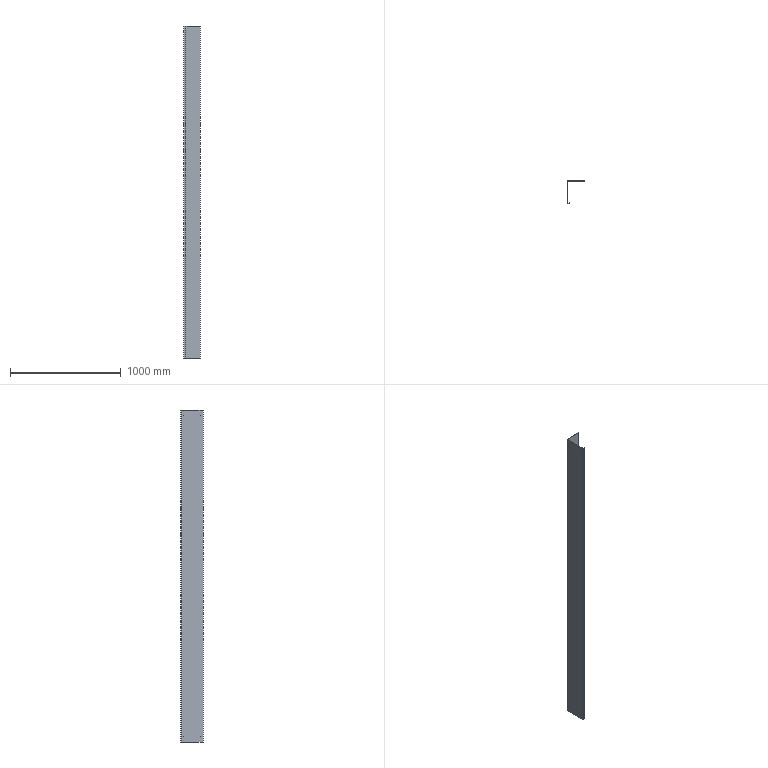Part | STEP file | TS-S50 | 1 solid | 30 faces | box 150.007 x 206.045 x 2995 mm | volume 2202698 mm3 | plane 18 | cylinder 12 | commonest cylinder face diameters 5.4 x8 0.4 x2 4.4 x2